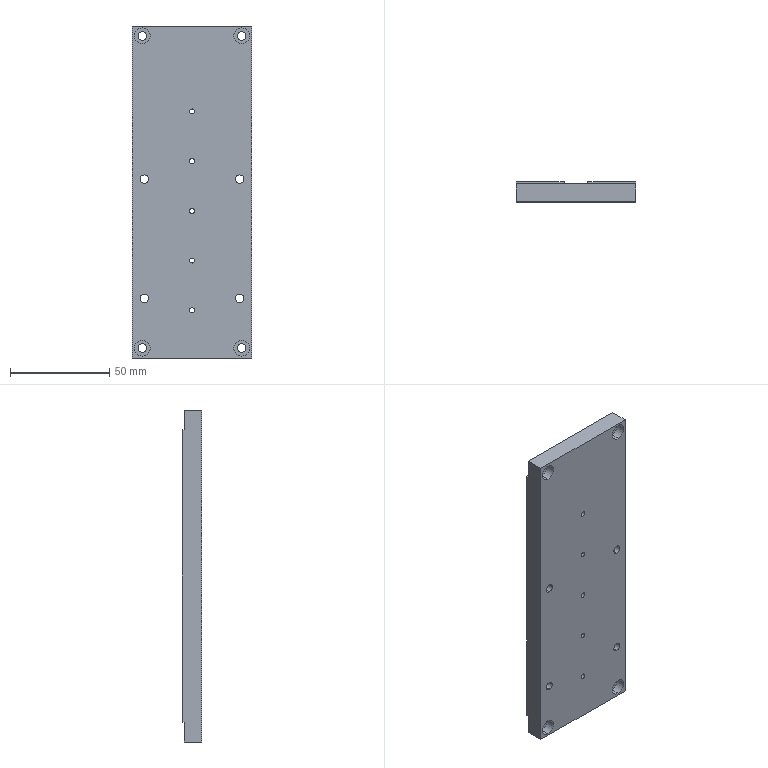Part | STEP file | 2075 Mounting base plate | 1 solid | 52 faces | box 60 x 10 x 167 mm | volume 95280 mm3 | cylinder 34 | plane 18 | commonest cylinder face diameters 2.5 x10 4.2 x8 4.3 x8 8 x8